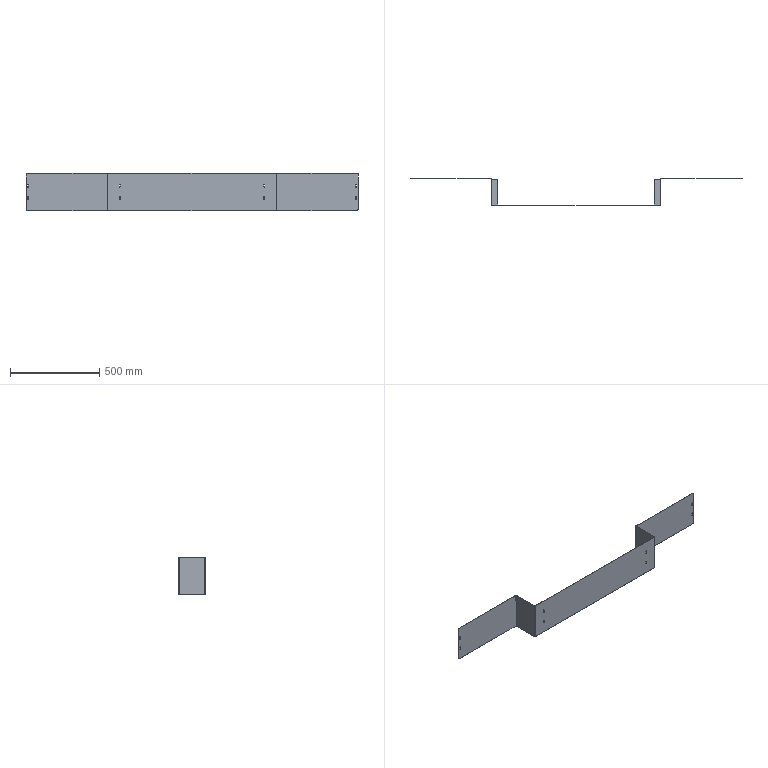Part | SolidWorks | features BaseBody 1 | 1 solid | 82 faces | box 1860 x 150 x 212.237 mm | volume 693950 mm3 | plane 42 | cylinder 40 | commonest cylinder face diameters 7 x24 1.473 x6 4.473 x6 10 x4